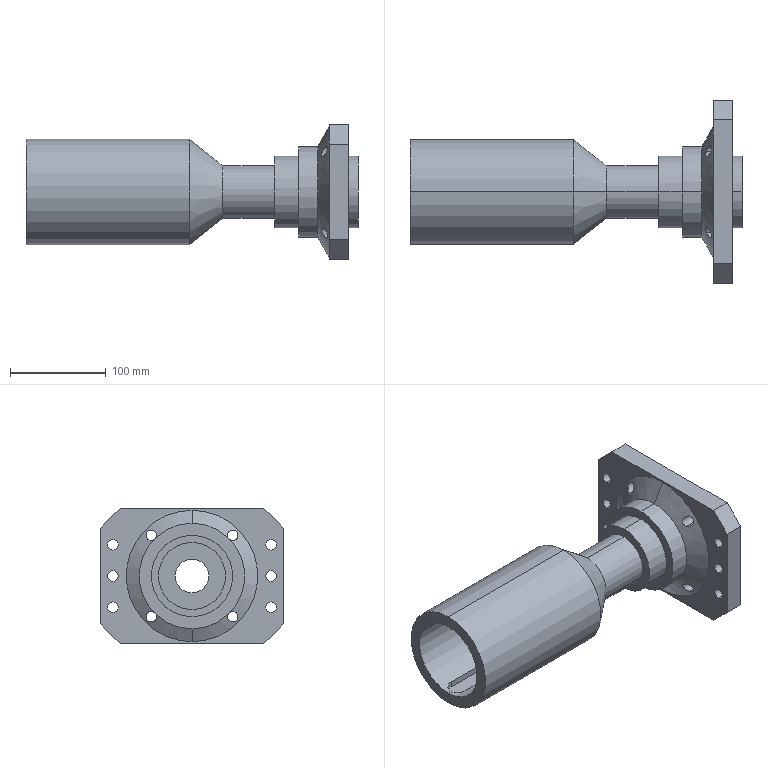Part | SolidWorks | features ICE 6, Revolution 2, RefAxis 1 | 1 solid | 71 faces | box 346 x 190 x 140 mm | volume 1651422 mm3 | cylinder 44 | plane 23 | cone 4 | commonest cylinder face diameters 11 x20 22 x6 75 x4 35 x2 42 x2 55 x2